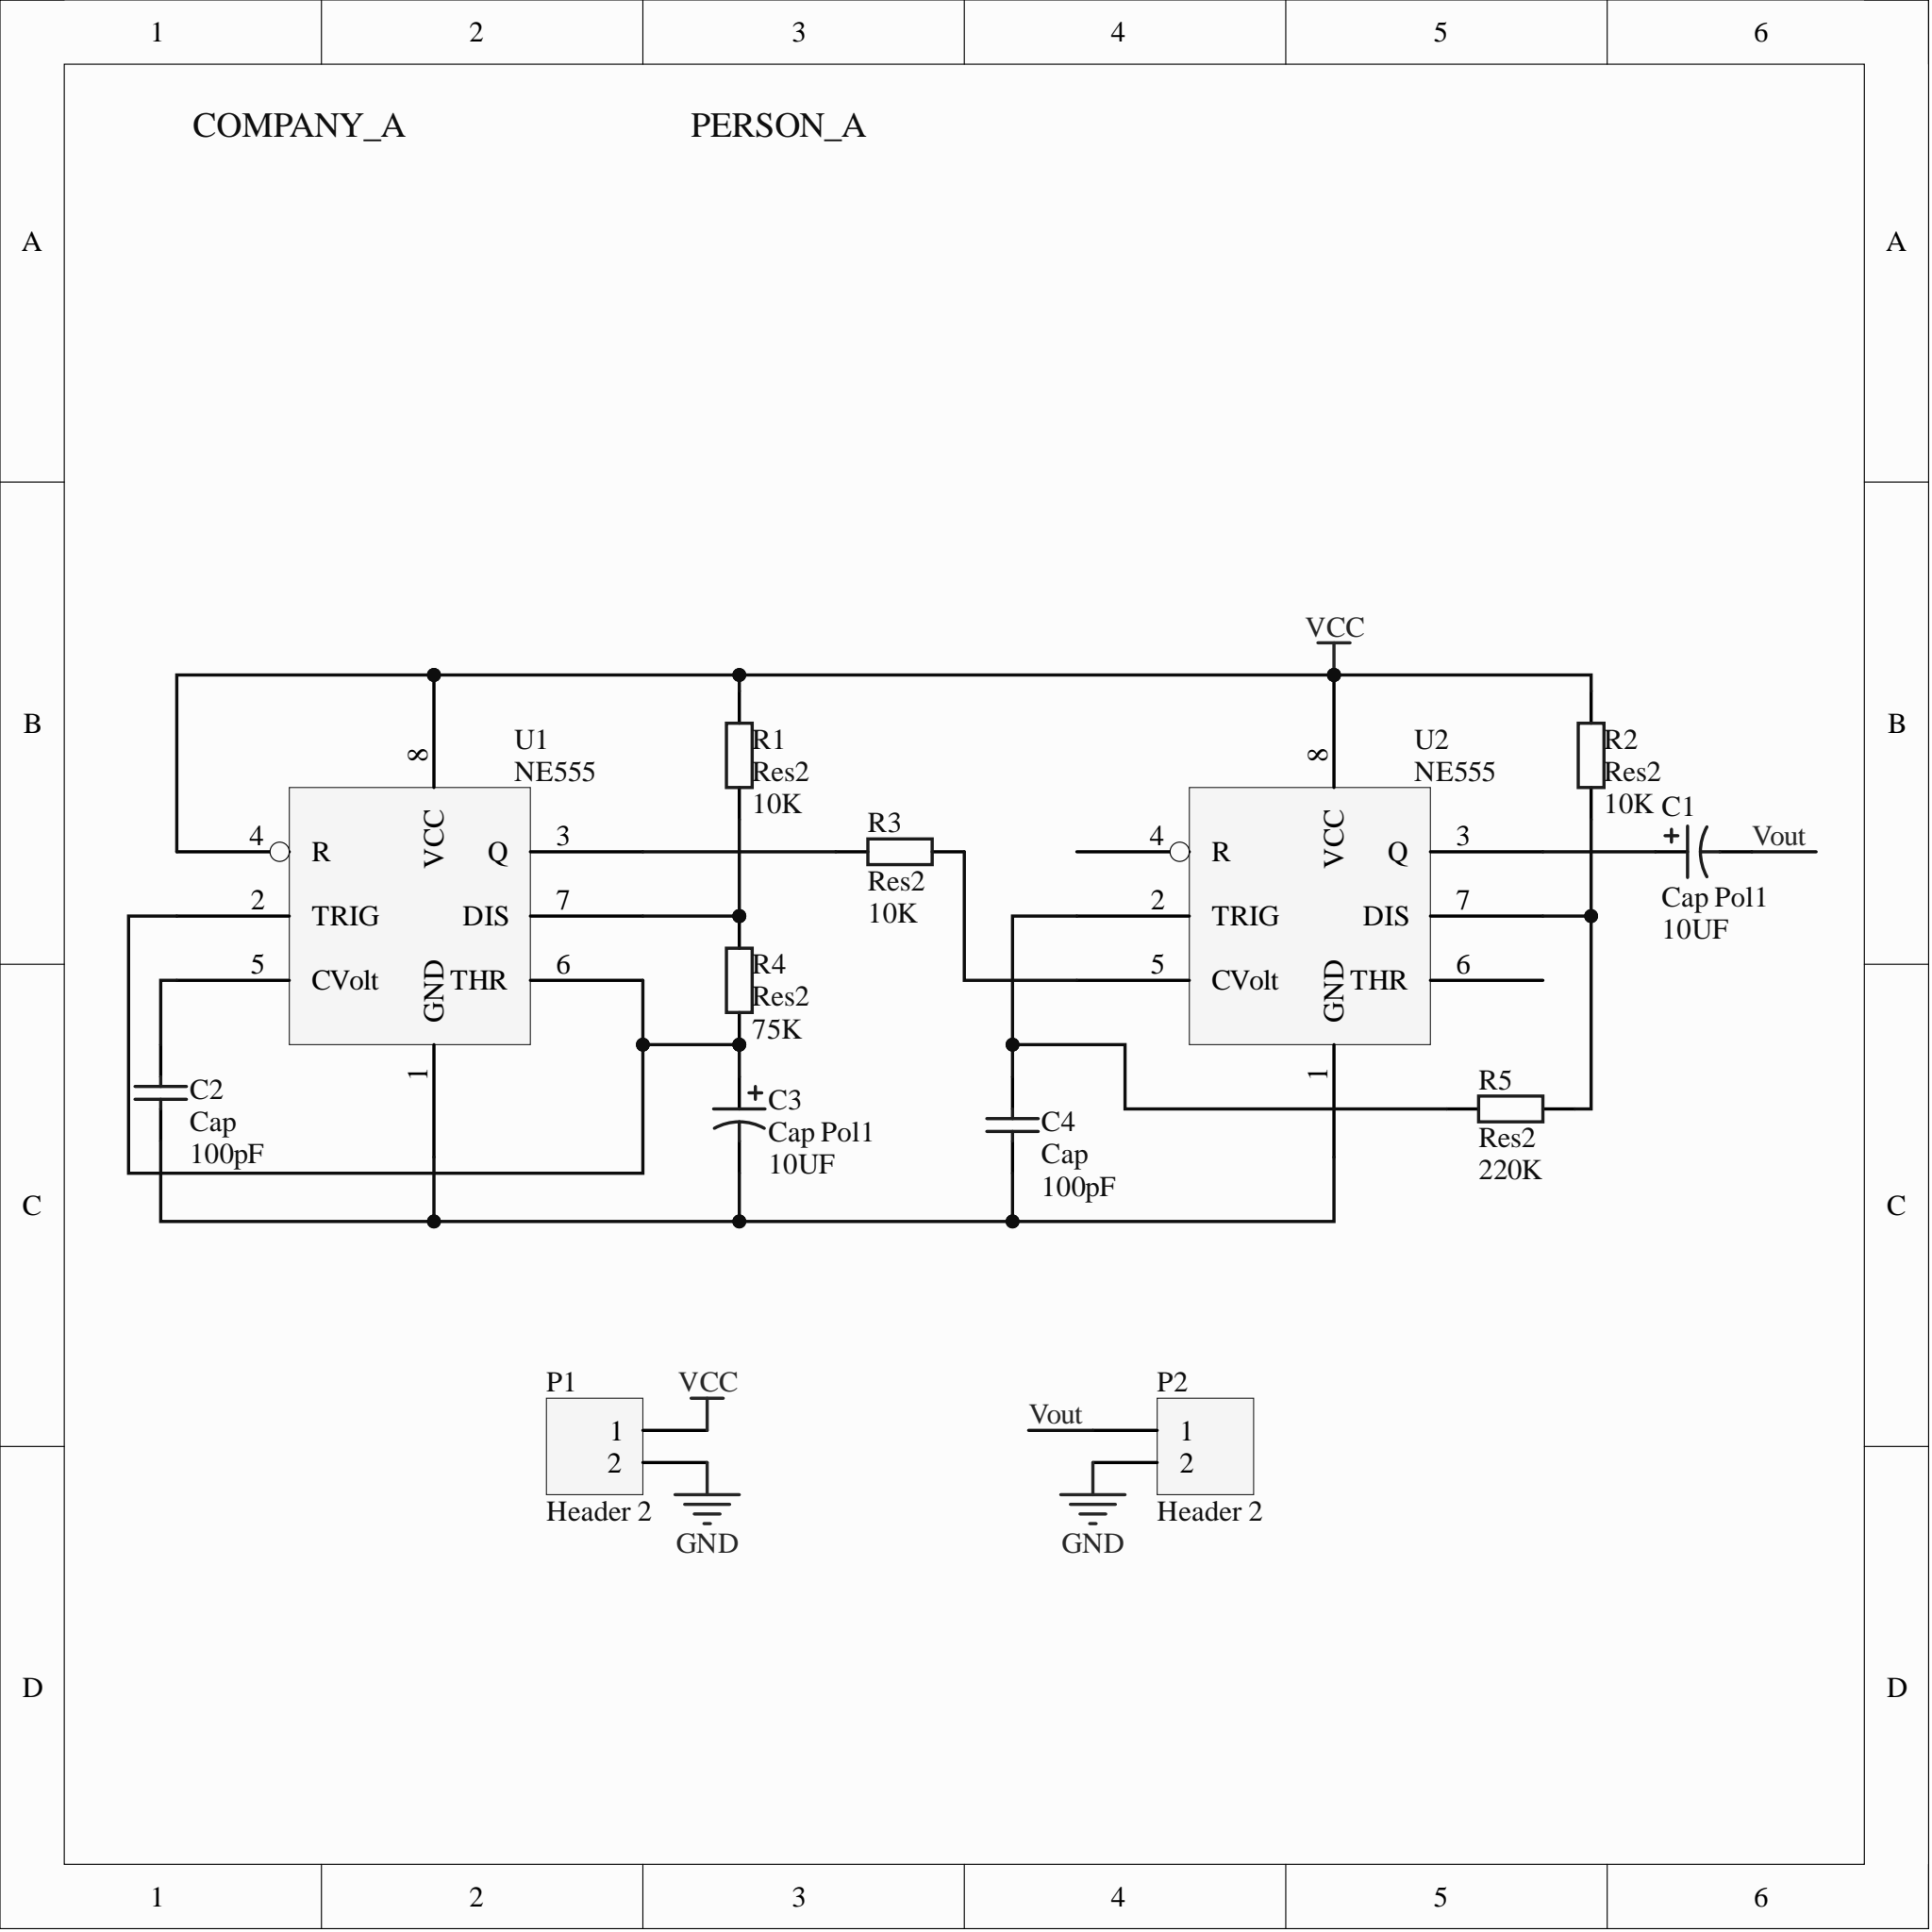Circuit board | Altium Designer | 13 parts | 12 nets
Bill of materials:
Comment,Description,Designator,Footprint,LibRef,Quantity
"Cap Pol1","Polarized Capacitor (Radial)","C1, C3","RB7.6-15","Cap Pol1","2"
"Cap","Capacitor","C2, C4","RAD-0.3","Cap","2"
"Header 2","Header, 2-Pin","P1, P2","HDR1X2","Header 2","2"
"Res2","Resistor","R1, R2, R3, R4, R5","AXIAL-0.4","Res2","5"
"NE555","","U1, U2","DIP8","NE555","2"
Netlist (Protel format):
[
C1
RB7.6-15
Cap Pol1



]
[
C2
RAD-0.3
Cap



]
[
C3
RB7.6-15
Cap Pol1



]
[
C4
RAD-0.3
Cap



]
[
P1
HDR1X2
Header 2



]
[
P2
HDR1X2
Header 2



]
[
R1
AXIAL-0.4
Res2



]
[
R2
AXIAL-0.4
Res2



]
[
R3
AXIAL-0.4
Res2



]
[
R4
AXIAL-0.4
Res2



]
[
R5
AXIAL-0.4
Res2



]
[
U1
DIP8
NE555



]
[
U2
DIP8
NE555



]
(
Vout
C1-2
P2-1
)
(
VCC
P1-1
R1-2
R2-2
U1-4
U1-8
U2-8
)
(
NetR3_2
R3-2
U1-3
)
(
NetR3_1
R3-1
U2-5
)
(
NetR2_1
R2-1
R5-1
U2-7
)
(
NetR1_1
R1-1
R4-2
U1-7
)
(
NetC4_2
C4-2
R5-2
U2-2
)
(
NetC3_1
C3-1
R4-1
U1-2
U1-6
)
(
NetC2_2
C2-2
U1-5
)
(
NetC2_1
C2-1
C3-2
C4-1
U1-1
U2-1
)
(
NetC1_1
C1-1
U2-3
)
(
GND
P1-2
P2-2
)